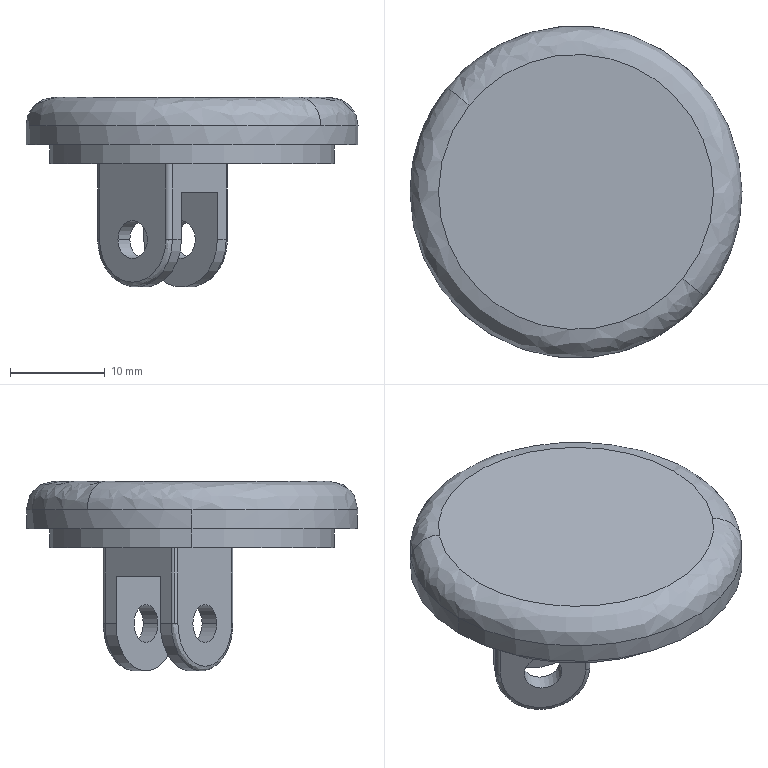Part | SolidWorks | features BaseBody 1 | 1 solid | 29 faces | box 35 x 35 x 20 mm | volume 6625 mm3 | cylinder 15 | plane 10 | spline 4 | commonest cylinder face diameters 1 x5 4 x4 10 x2 30 x2 35 x2